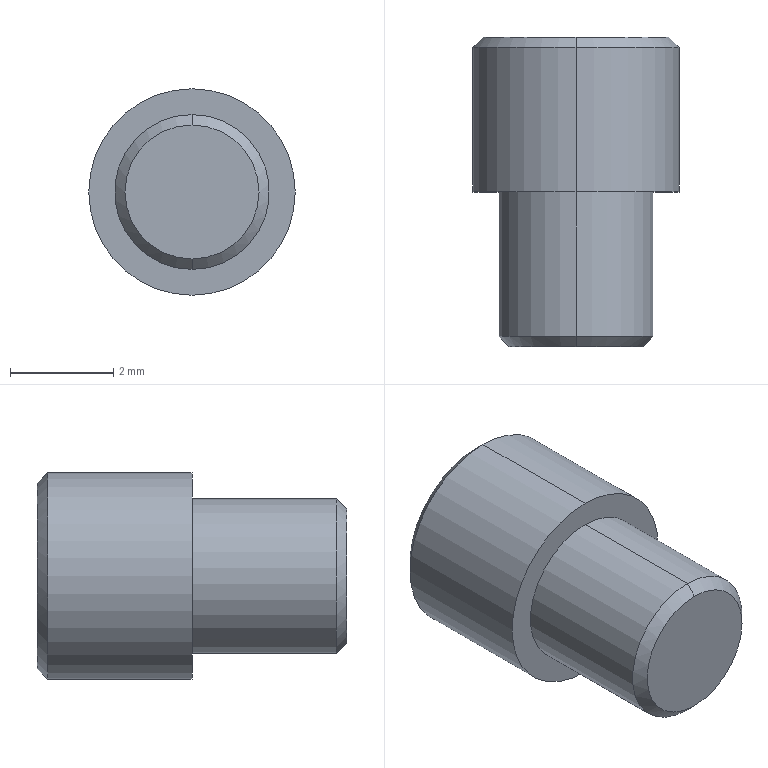Part | SolidWorks | features Chamfer 1, Extrusion 1, ICE 1 | 1 solid | 11 faces | box 4 x 6 x 4 mm | volume 58.482 mm3 | cone 4 | cylinder 4 | plane 3 | commonest cylinder face diameters 3 x2 4 x2
STEP:
#1=CARTESIAN_POINT('',(0.,0.,-1.3));
#2=VERTEX_POINT('',#1);
#3=CARTESIAN_POINT('',(0.,0.,1.3));
#4=VERTEX_POINT('',#3);
#5=CARTESIAN_POINT('',(0.,0.,0.));
#6=DIRECTION('',(0.,-1.,0.));
#7=DIRECTION('',(0.,0.,1.));
#8=AXIS2_PLACEMENT_3D('',#5,#6,#7);
#9=CIRCLE('',#8,1.3);
#10=EDGE_CURVE('',#2,#4,#9,.T.);
#11=ORIENTED_EDGE('',*,*,#10,.F.);
#12=CARTESIAN_POINT('',(0.,0.2,-1.5));
#13=VERTEX_POINT('',#12);
#14=CARTESIAN_POINT('',(0.,0.2,-1.5));
#15=DIRECTION('',(0.,0.7071,-0.7071));
#16=VECTOR('',#15,1000.);
#17=LINE('',#14,#16);
#18=EDGE_CURVE('',#2,#13,#17,.T.);
#19=ORIENTED_EDGE('',*,*,#18,.T.);
#20=CARTESIAN_POINT('',(0.,0.2,1.5));
#21=VERTEX_POINT('',#20);
#22=CARTESIAN_POINT('',(0.,0.2,0.));
#23=DIRECTION('',(0.,1.,0.));
#24=DIRECTION('',(0.,0.,1.));
#25=AXIS2_PLACEMENT_3D('',#22,#23,#24);
#26=CIRCLE('',#25,1.5);
#27=EDGE_CURVE('',#21,#13,#26,.T.);
#28=ORIENTED_EDGE('',*,*,#27,.F.);
#29=CARTESIAN_POINT('',(0.,0.2,1.5));
#30=DIRECTION('',(0.,0.7071,0.7071));
#31=VECTOR('',#30,1000.);
#32=LINE('',#29,#31);
#33=EDGE_CURVE('',#4,#21,#32,.T.);
#34=ORIENTED_EDGE('',*,*,#33,.F.);
#35=EDGE_LOOP('',(#11,#19,#28,#34));
#36=FACE_OUTER_BOUND('',#35,.T.);
#37=CARTESIAN_POINT('',(0.,0.2,0.));
#38=DIRECTION('',(0.,1.,0.));
#39=DIRECTION('',(0.,0.,1.));
#40=AXIS2_PLACEMENT_3D('',#37,#38,#39);
#41=CONICAL_SURFACE('',#40,1.5,0.7854);
#42=ADVANCED_FACE('',(#36),#41,.T.);
#43=CARTESIAN_POINT('',(0.,6.,1.8));
#44=VERTEX_POINT('',#43);
#45=CARTESIAN_POINT('',(0.,6.,-1.8));
#46=VERTEX_POINT('',#45);
#47=CARTESIAN_POINT('',(0.,6.,0.));
#48=DIRECTION('',(0.,1.,0.));
#49=DIRECTION('',(0.,0.,1.));
#50=AXIS2_PLACEMENT_3D('',#47,#48,#49);
#51=CIRCLE('',#50,1.8);
#52=EDGE_CURVE('',#44,#46,#51,.T.);
#53=ORIENTED_EDGE('',*,*,#52,.F.);
#54=CARTESIAN_POINT('',(0.,5.8,2.));
#55=VERTEX_POINT('',#54);
#56=CARTESIAN_POINT('',(0.,6.,1.8));
#57=DIRECTION('',(0.,-0.7071,0.7071));
#58=VECTOR('',#57,1000.);
#59=LINE('',#56,#58);
#60=EDGE_CURVE('',#44,#55,#59,.T.);
#61=ORIENTED_EDGE('',*,*,#60,.T.);
#62=CARTESIAN_POINT('',(0.,5.8,-2.));
#63=VERTEX_POINT('',#62);
#64=CARTESIAN_POINT('',(0.,5.8,0.));
#65=DIRECTION('',(0.,-1.,0.));
#66=DIRECTION('',(0.,0.,1.));
#67=AXIS2_PLACEMENT_3D('',#64,#65,#66);
#68=CIRCLE('',#67,2.);
#69=EDGE_CURVE('',#63,#55,#68,.T.);
#70=ORIENTED_EDGE('',*,*,#69,.F.);
#71=CARTESIAN_POINT('',(0.,6.,-1.8));
#72=DIRECTION('',(0.,-0.7071,-0.7071));
#73=VECTOR('',#72,1000.);
#74=LINE('',#71,#73);
#75=EDGE_CURVE('',#46,#63,#74,.T.);
#76=ORIENTED_EDGE('',*,*,#75,.F.);
#77=EDGE_LOOP('',(#53,#61,#70,#76));
#78=FACE_OUTER_BOUND('',#77,.T.);
#79=CARTESIAN_POINT('',(0.,6.,0.));
#80=DIRECTION('',(0.,-1.,0.));
#81=DIRECTION('',(0.,0.,-1.));
#82=AXIS2_PLACEMENT_3D('',#79,#80,#81);
#83=CONICAL_SURFACE('',#82,1.8,0.7854);
#84=ADVANCED_FACE('',(#78),#83,.T.);
#85=ORIENTED_EDGE('',*,*,#69,.T.);
#86=CARTESIAN_POINT('',(0.,3.,2.));
#87=VERTEX_POINT('',#86);
#88=CARTESIAN_POINT('',(0.,6.,2.));
#89=DIRECTION('',(0.,-1.,0.));
#90=VECTOR('',#89,1000.);
#91=LINE('',#88,#90);
#92=EDGE_CURVE('',#55,#87,#91,.T.);
#93=ORIENTED_EDGE('',*,*,#92,.T.);
#94=CARTESIAN_POINT('',(0.,3.,-2.));
#95=VERTEX_POINT('',#94);
#96=CARTESIAN_POINT('',(0.,3.,0.));
#97=DIRECTION('',(0.,1.,0.));
#98=DIRECTION('',(0.,0.,1.));
#99=AXIS2_PLACEMENT_3D('',#96,#97,#98);
#100=CIRCLE('',#99,2.);
#101=EDGE_CURVE('',#87,#95,#100,.T.);
#102=ORIENTED_EDGE('',*,*,#101,.T.);
#103=CARTESIAN_POINT('',(0.,6.,-2.));
#104=DIRECTION('',(0.,-1.,0.));
#105=VECTOR('',#104,1000.);
#106=LINE('',#103,#105);
#107=EDGE_CURVE('',#63,#95,#106,.T.);
#108=ORIENTED_EDGE('',*,*,#107,.F.);
#109=EDGE_LOOP('',(#85,#93,#102,#108));
#110=FACE_OUTER_BOUND('',#109,.T.);
#111=CARTESIAN_POINT('',(0.,6.,0.));
#112=DIRECTION('',(0.,-1.,0.));
#113=DIRECTION('',(0.,0.,-1.));
#114=AXIS2_PLACEMENT_3D('',#111,#112,#113);
#115=CYLINDRICAL_SURFACE('',#114,2.);
#116=ADVANCED_FACE('',(#110),#115,.T.);
#117=CARTESIAN_POINT('',(0.,3.,1.5));
#118=VERTEX_POINT('',#117);
#119=CARTESIAN_POINT('',(0.,3.,-1.5));
#120=VERTEX_POINT('',#119);
#121=CARTESIAN_POINT('',(0.,3.,0.));
#122=DIRECTION('',(0.,1.,0.));
#123=DIRECTION('',(0.,0.,1.));
#124=AXIS2_PLACEMENT_3D('',#121,#122,#123);
#125=CIRCLE('',#124,1.5);
#126=EDGE_CURVE('',#118,#120,#125,.T.);
#127=ORIENTED_EDGE('',*,*,#126,.F.);
#128=CARTESIAN_POINT('',(0.,3.,1.5));
#129=DIRECTION('',(0.,-1.,0.));
#130=VECTOR('',#129,1000.);
#131=LINE('',#128,#130);
#132=EDGE_CURVE('',#118,#21,#131,.T.);
#133=ORIENTED_EDGE('',*,*,#132,.T.);
#134=ORIENTED_EDGE('',*,*,#27,.T.);
#135=CARTESIAN_POINT('',(0.,3.,-1.5));
#136=DIRECTION('',(0.,-1.,0.));
#137=VECTOR('',#136,1000.);
#138=LINE('',#135,#137);
#139=EDGE_CURVE('',#120,#13,#138,.T.);
#140=ORIENTED_EDGE('',*,*,#139,.F.);
#141=EDGE_LOOP('',(#127,#133,#134,#140));
#142=FACE_OUTER_BOUND('',#141,.T.);
#143=CARTESIAN_POINT('',(0.,3.,0.));
#144=DIRECTION('',(0.,-1.,0.));
#145=DIRECTION('',(0.,0.,-1.));
#146=AXIS2_PLACEMENT_3D('',#143,#144,#145);
#147=CYLINDRICAL_SURFACE('',#146,1.5);
#148=ADVANCED_FACE('',(#142),#147,.T.);
#149=ORIENTED_EDGE('',*,*,#132,.F.);
#150=CARTESIAN_POINT('',(0.,3.,0.));
#151=DIRECTION('',(0.,1.,0.));
#152=DIRECTION('',(0.,0.,1.));
#153=AXIS2_PLACEMENT_3D('',#150,#151,#152);
#154=CIRCLE('',#153,1.5);
#155=EDGE_CURVE('',#120,#118,#154,.T.);
#156=ORIENTED_EDGE('',*,*,#155,.F.);
#157=ORIENTED_EDGE('',*,*,#139,.T.);
#158=CARTESIAN_POINT('',(0.,0.2,0.));
#159=DIRECTION('',(0.,1.,0.));
#160=DIRECTION('',(0.,0.,1.));
#161=AXIS2_PLACEMENT_3D('',#158,#159,#160);
#162=CIRCLE('',#161,1.5);
#163=EDGE_CURVE('',#13,#21,#162,.T.);
#164=ORIENTED_EDGE('',*,*,#163,.T.);
#165=EDGE_LOOP('',(#149,#156,#157,#164));
#166=FACE_OUTER_BOUND('',#165,.T.);
#167=CARTESIAN_POINT('',(0.,3.,0.));
#168=DIRECTION('',(0.,-1.,0.));
#169=DIRECTION('',(0.,0.,-1.));
#170=AXIS2_PLACEMENT_3D('',#167,#168,#169);
#171=CYLINDRICAL_SURFACE('',#170,1.5);
#172=ADVANCED_FACE('',(#166),#171,.T.);
#173=CARTESIAN_POINT('',(0.,0.,0.));
#174=DIRECTION('',(0.,-1.,0.));
#175=DIRECTION('',(0.,0.,1.));
#176=AXIS2_PLACEMENT_3D('',#173,#174,#175);
#177=CIRCLE('',#176,1.3);
#178=EDGE_CURVE('',#4,#2,#177,.T.);
#179=ORIENTED_EDGE('',*,*,#178,.T.);
#180=ORIENTED_EDGE('',*,*,#10,.T.);
#181=EDGE_LOOP('',(#179,#180));
#182=FACE_OUTER_BOUND('',#181,.T.);
#183=CARTESIAN_POINT('',(0.,0.,0.));
#184=DIRECTION('',(0.,1.,0.));
#185=DIRECTION('',(0.,0.,1.));
#186=AXIS2_PLACEMENT_3D('',#183,#184,#185);
#187=PLANE('',#186);
#188=ADVANCED_FACE('',(#182),#187,.F.);
#189=CARTESIAN_POINT('',(0.,3.,0.));
#190=DIRECTION('',(0.,1.,0.));
#191=DIRECTION('',(0.,0.,1.));
#192=AXIS2_PLACEMENT_3D('',#189,#190,#191);
#193=CIRCLE('',#192,2.);
#194=EDGE_CURVE('',#95,#87,#193,.T.);
#195=ORIENTED_EDGE('',*,*,#194,.F.);
#196=ORIENTED_EDGE('',*,*,#101,.F.);
#197=EDGE_LOOP('',(#195,#196));
#198=FACE_OUTER_BOUND('',#197,.T.);
#199=ORIENTED_EDGE('',*,*,#155,.T.);
#200=ORIENTED_EDGE('',*,*,#126,.T.);
#201=EDGE_LOOP('',(#199,#200));
#202=FACE_BOUND('',#201,.T.);
#203=CARTESIAN_POINT('',(0.,3.,0.));
#204=DIRECTION('',(0.,1.,0.));
#205=DIRECTION('',(0.,0.,1.));
#206=AXIS2_PLACEMENT_3D('',#203,#204,#205);
#207=PLANE('',#206);
#208=ADVANCED_FACE('',(#198,#202),#207,.F.);
#209=ORIENTED_EDGE('',*,*,#92,.F.);
#210=CARTESIAN_POINT('',(0.,5.8,0.));
#211=DIRECTION('',(0.,-1.,0.));
#212=DIRECTION('',(0.,0.,1.));
#213=AXIS2_PLACEMENT_3D('',#210,#211,#212);
#214=CIRCLE('',#213,2.);
#215=EDGE_CURVE('',#55,#63,#214,.T.);
#216=ORIENTED_EDGE('',*,*,#215,.T.);
#217=ORIENTED_EDGE('',*,*,#107,.T.);
#218=ORIENTED_EDGE('',*,*,#194,.T.);
#219=EDGE_LOOP('',(#209,#216,#217,#218));
#220=FACE_OUTER_BOUND('',#219,.T.);
#221=CARTESIAN_POINT('',(0.,6.,0.));
#222=DIRECTION('',(0.,-1.,0.));
#223=DIRECTION('',(0.,0.,-1.));
#224=AXIS2_PLACEMENT_3D('',#221,#222,#223);
#225=CYLINDRICAL_SURFACE('',#224,2.);
#226=ADVANCED_FACE('',(#220),#225,.T.);
#227=CARTESIAN_POINT('',(0.,6.,0.));
#228=DIRECTION('',(0.,1.,0.));
#229=DIRECTION('',(0.,0.,1.));
#230=AXIS2_PLACEMENT_3D('',#227,#228,#229);
#231=CIRCLE('',#230,1.8);
#232=EDGE_CURVE('',#46,#44,#231,.T.);
#233=ORIENTED_EDGE('',*,*,#232,.T.);
#234=ORIENTED_EDGE('',*,*,#52,.T.);
#235=EDGE_LOOP('',(#233,#234));
#236=FACE_OUTER_BOUND('',#235,.T.);
#237=CARTESIAN_POINT('',(0.,6.,0.));
#238=DIRECTION('',(0.,1.,0.));
#239=DIRECTION('',(0.,0.,1.));
#240=AXIS2_PLACEMENT_3D('',#237,#238,#239);
#241=PLANE('',#240);
#242=ADVANCED_FACE('',(#236),#241,.T.);
#243=ORIENTED_EDGE('',*,*,#60,.F.);
#244=ORIENTED_EDGE('',*,*,#232,.F.);
#245=ORIENTED_EDGE('',*,*,#75,.T.);
#246=ORIENTED_EDGE('',*,*,#215,.F.);
#247=EDGE_LOOP('',(#243,#244,#245,#246));
#248=FACE_OUTER_BOUND('',#247,.T.);
#249=CARTESIAN_POINT('',(0.,6.,0.));
#250=DIRECTION('',(0.,-1.,0.));
#251=DIRECTION('',(0.,0.,-1.));
#252=AXIS2_PLACEMENT_3D('',#249,#250,#251);
#253=CONICAL_SURFACE('',#252,1.8,0.7854);
#254=ADVANCED_FACE('',(#248),#253,.T.);
#255=ORIENTED_EDGE('',*,*,#18,.F.);
#256=ORIENTED_EDGE('',*,*,#178,.F.);
#257=ORIENTED_EDGE('',*,*,#33,.T.);
#258=ORIENTED_EDGE('',*,*,#163,.F.);
#259=EDGE_LOOP('',(#255,#256,#257,#258));
#260=FACE_OUTER_BOUND('',#259,.T.);
#261=CARTESIAN_POINT('',(0.,0.2,0.));
#262=DIRECTION('',(0.,1.,0.));
#263=DIRECTION('',(0.,0.,1.));
#264=AXIS2_PLACEMENT_3D('',#261,#262,#263);
#265=CONICAL_SURFACE('',#264,1.5,0.7854);
#266=ADVANCED_FACE('',(#260),#265,.T.);
#267=CLOSED_SHELL('',(#42,#84,#116,#148,#172,#188,#208,#226,#242,#254,#266));
#268=MANIFOLD_SOLID_BREP('',#267);
#269=CARTESIAN_POINT('',(0.,0.,0.));
#270=DIRECTION('',(0.,0.,1.));
#271=DIRECTION('',(1.,0.,0.));
#272=AXIS2_PLACEMENT_3D('',#269,#270,#271);
#273=(LENGTH_UNIT()NAMED_UNIT(*)SI_UNIT(.MILLI.,.METRE.));
#274=UNCERTAINTY_MEASURE_WITH_UNIT(LENGTH_MEASURE(0.00001),#273,'','');
#275=(NAMED_UNIT(*)PLANE_ANGLE_UNIT()SI_UNIT($,.RADIAN.));
#276=(NAMED_UNIT(*)SI_UNIT($,.STERADIAN.)SOLID_ANGLE_UNIT());
#277=(GEOMETRIC_REPRESENTATION_CONTEXT(3)GLOBAL_UNCERTAINTY_ASSIGNED_CONTEXT((#274))GLOBAL_UNIT_ASSIGNED_CONTEXT((#273,#275,#276))REPRESENTATION_CONTEXT('',''));
#278=ADVANCED_BREP_SHAPE_REPRESENTATION('',(#268,#272),#277);